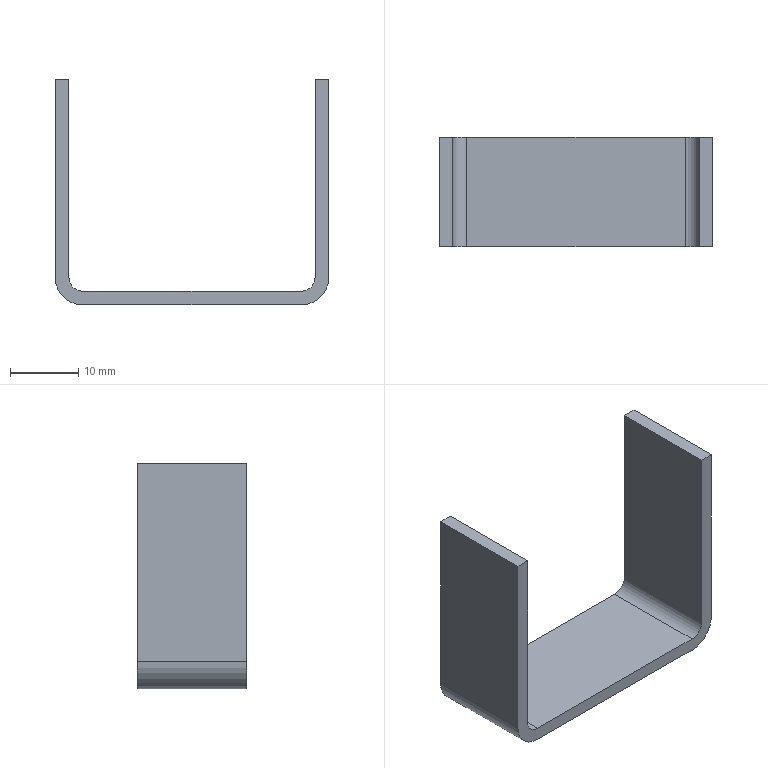Part | NX | features solid 2 | 1 solid | 14 faces | box 40 x 16 x 33 mm | volume 3182 mm3 | plane 10 | cylinder 4 | commonest cylinder face diameters 4 x2 8 x2
STEP:
#1=CARTESIAN_POINT('',(941.4,-1578.,922.));
#2=VERTEX_POINT('',#1);
#3=CARTESIAN_POINT('',(941.4,-1578.,951.));
#4=VERTEX_POINT('',#3);
#5=CARTESIAN_POINT('',(941.4,-1578.,918.));
#6=DIRECTION('',(0.,0.,1.));
#7=VECTOR('',#6,1000.);
#8=LINE('',#5,#7);
#9=EDGE_CURVE('',#2,#4,#8,.T.);
#10=ORIENTED_EDGE('',*,*,#9,.T.);
#11=CARTESIAN_POINT('',(941.4,-1562.,951.));
#12=VERTEX_POINT('',#11);
#13=CARTESIAN_POINT('',(941.4,-1562.,951.));
#14=DIRECTION('',(0.,-1.,0.));
#15=VECTOR('',#14,1000.);
#16=LINE('',#13,#15);
#17=EDGE_CURVE('',#12,#4,#16,.T.);
#18=ORIENTED_EDGE('',*,*,#17,.F.);
#19=CARTESIAN_POINT('',(941.4,-1562.,922.));
#20=VERTEX_POINT('',#19);
#21=CARTESIAN_POINT('',(941.4,-1562.,918.));
#22=DIRECTION('',(0.,0.,1.));
#23=VECTOR('',#22,1000.);
#24=LINE('',#21,#23);
#25=EDGE_CURVE('',#20,#12,#24,.T.);
#26=ORIENTED_EDGE('',*,*,#25,.F.);
#27=CARTESIAN_POINT('',(941.4,-1562.,922.));
#28=DIRECTION('',(0.,-1.,0.));
#29=VECTOR('',#28,1000.);
#30=LINE('',#27,#29);
#31=EDGE_CURVE('',#20,#2,#30,.T.);
#32=ORIENTED_EDGE('',*,*,#31,.T.);
#33=EDGE_LOOP('',(#10,#18,#26,#32));
#34=FACE_BOUND('',#33,.T.);
#35=CARTESIAN_POINT('',(941.4,-1562.,918.));
#36=DIRECTION('',(1.,0.,0.));
#37=DIRECTION('',(0.,1.,0.));
#38=AXIS2_PLACEMENT_3D('',#35,#36,#37);
#39=PLANE('',#38);
#40=ADVANCED_FACE('',(#34),#39,.F.);
#41=CARTESIAN_POINT('',(939.4,-1578.,920.));
#42=VERTEX_POINT('',#41);
#43=CARTESIAN_POINT('',(939.4,-1578.,922.));
#44=DIRECTION('',(0.,-1.,0.));
#45=DIRECTION('',(0.,0.,-1.));
#46=AXIS2_PLACEMENT_3D('',#43,#44,#45);
#47=CIRCLE('',#46,2.);
#48=EDGE_CURVE('',#42,#2,#47,.T.);
#49=ORIENTED_EDGE('',*,*,#48,.T.);
#50=ORIENTED_EDGE('',*,*,#31,.F.);
#51=CARTESIAN_POINT('',(939.4,-1562.,920.));
#52=VERTEX_POINT('',#51);
#53=CARTESIAN_POINT('',(939.4,-1562.,922.));
#54=DIRECTION('',(0.,-1.,0.));
#55=DIRECTION('',(0.,0.,-1.));
#56=AXIS2_PLACEMENT_3D('',#53,#54,#55);
#57=CIRCLE('',#56,2.);
#58=EDGE_CURVE('',#52,#20,#57,.T.);
#59=ORIENTED_EDGE('',*,*,#58,.F.);
#60=CARTESIAN_POINT('',(939.4,-1562.,920.));
#61=DIRECTION('',(0.,-1.,0.));
#62=VECTOR('',#61,1000.);
#63=LINE('',#60,#62);
#64=EDGE_CURVE('',#52,#42,#63,.T.);
#65=ORIENTED_EDGE('',*,*,#64,.T.);
#66=EDGE_LOOP('',(#49,#50,#59,#65));
#67=FACE_BOUND('',#66,.T.);
#68=CARTESIAN_POINT('',(939.4,-1562.,922.));
#69=DIRECTION('',(0.,-1.,0.));
#70=DIRECTION('',(0.,0.,-1.));
#71=AXIS2_PLACEMENT_3D('',#68,#69,#70);
#72=CYLINDRICAL_SURFACE('',#71,2.);
#73=ADVANCED_FACE('',(#67),#72,.F.);
#74=CARTESIAN_POINT('',(907.4,-1578.,920.));
#75=VERTEX_POINT('',#74);
#76=CARTESIAN_POINT('',(903.4,-1578.,920.));
#77=DIRECTION('',(1.,0.,0.));
#78=VECTOR('',#77,1000.);
#79=LINE('',#76,#78);
#80=EDGE_CURVE('',#75,#42,#79,.T.);
#81=ORIENTED_EDGE('',*,*,#80,.T.);
#82=ORIENTED_EDGE('',*,*,#64,.F.);
#83=CARTESIAN_POINT('',(907.4,-1562.,920.));
#84=VERTEX_POINT('',#83);
#85=CARTESIAN_POINT('',(903.4,-1562.,920.));
#86=DIRECTION('',(1.,0.,0.));
#87=VECTOR('',#86,1000.);
#88=LINE('',#85,#87);
#89=EDGE_CURVE('',#84,#52,#88,.T.);
#90=ORIENTED_EDGE('',*,*,#89,.F.);
#91=CARTESIAN_POINT('',(907.4,-1562.,920.));
#92=DIRECTION('',(0.,-1.,0.));
#93=VECTOR('',#92,1000.);
#94=LINE('',#91,#93);
#95=EDGE_CURVE('',#84,#75,#94,.T.);
#96=ORIENTED_EDGE('',*,*,#95,.T.);
#97=EDGE_LOOP('',(#81,#82,#90,#96));
#98=FACE_BOUND('',#97,.T.);
#99=CARTESIAN_POINT('',(903.4,-1562.,920.));
#100=DIRECTION('',(0.,0.,-1.));
#101=DIRECTION('',(0.,-1.,0.));
#102=AXIS2_PLACEMENT_3D('',#99,#100,#101);
#103=PLANE('',#102);
#104=ADVANCED_FACE('',(#98),#103,.F.);
#105=CARTESIAN_POINT('',(905.4,-1578.,922.));
#106=VERTEX_POINT('',#105);
#107=CARTESIAN_POINT('',(907.4,-1578.,922.));
#108=DIRECTION('',(0.,-1.,0.));
#109=DIRECTION('',(0.,0.,-1.));
#110=AXIS2_PLACEMENT_3D('',#107,#108,#109);
#111=CIRCLE('',#110,2.);
#112=EDGE_CURVE('',#106,#75,#111,.T.);
#113=ORIENTED_EDGE('',*,*,#112,.T.);
#114=ORIENTED_EDGE('',*,*,#95,.F.);
#115=CARTESIAN_POINT('',(905.4,-1562.,922.));
#116=VERTEX_POINT('',#115);
#117=CARTESIAN_POINT('',(907.4,-1562.,922.));
#118=DIRECTION('',(0.,-1.,0.));
#119=DIRECTION('',(0.,0.,-1.));
#120=AXIS2_PLACEMENT_3D('',#117,#118,#119);
#121=CIRCLE('',#120,2.);
#122=EDGE_CURVE('',#116,#84,#121,.T.);
#123=ORIENTED_EDGE('',*,*,#122,.F.);
#124=CARTESIAN_POINT('',(905.4,-1562.,922.));
#125=DIRECTION('',(0.,-1.,0.));
#126=VECTOR('',#125,1000.);
#127=LINE('',#124,#126);
#128=EDGE_CURVE('',#116,#106,#127,.T.);
#129=ORIENTED_EDGE('',*,*,#128,.T.);
#130=EDGE_LOOP('',(#113,#114,#123,#129));
#131=FACE_BOUND('',#130,.T.);
#132=CARTESIAN_POINT('',(907.4,-1562.,922.));
#133=DIRECTION('',(0.,-1.,0.));
#134=DIRECTION('',(0.,0.,-1.));
#135=AXIS2_PLACEMENT_3D('',#132,#133,#134);
#136=CYLINDRICAL_SURFACE('',#135,2.);
#137=ADVANCED_FACE('',(#131),#136,.F.);
#138=CARTESIAN_POINT('',(905.4,-1578.,951.));
#139=VERTEX_POINT('',#138);
#140=CARTESIAN_POINT('',(905.4,-1578.,951.));
#141=DIRECTION('',(0.,0.,-1.));
#142=VECTOR('',#141,1000.);
#143=LINE('',#140,#142);
#144=EDGE_CURVE('',#139,#106,#143,.T.);
#145=ORIENTED_EDGE('',*,*,#144,.T.);
#146=ORIENTED_EDGE('',*,*,#128,.F.);
#147=CARTESIAN_POINT('',(905.4,-1562.,951.));
#148=VERTEX_POINT('',#147);
#149=CARTESIAN_POINT('',(905.4,-1562.,951.));
#150=DIRECTION('',(0.,0.,-1.));
#151=VECTOR('',#150,1000.);
#152=LINE('',#149,#151);
#153=EDGE_CURVE('',#148,#116,#152,.T.);
#154=ORIENTED_EDGE('',*,*,#153,.F.);
#155=CARTESIAN_POINT('',(905.4,-1562.,951.));
#156=DIRECTION('',(0.,-1.,0.));
#157=VECTOR('',#156,1000.);
#158=LINE('',#155,#157);
#159=EDGE_CURVE('',#148,#139,#158,.T.);
#160=ORIENTED_EDGE('',*,*,#159,.T.);
#161=EDGE_LOOP('',(#145,#146,#154,#160));
#162=FACE_BOUND('',#161,.T.);
#163=CARTESIAN_POINT('',(905.4,-1562.,951.));
#164=DIRECTION('',(-1.,0.,0.));
#165=DIRECTION('',(0.,0.,1.));
#166=AXIS2_PLACEMENT_3D('',#163,#164,#165);
#167=PLANE('',#166);
#168=ADVANCED_FACE('',(#162),#167,.F.);
#169=CARTESIAN_POINT('',(943.4,-1578.,922.));
#170=VERTEX_POINT('',#169);
#171=CARTESIAN_POINT('',(943.4,-1578.,951.));
#172=VERTEX_POINT('',#171);
#173=CARTESIAN_POINT('',(943.4,-1578.,918.));
#174=DIRECTION('',(0.,0.,1.));
#175=VECTOR('',#174,1000.);
#176=LINE('',#173,#175);
#177=EDGE_CURVE('',#170,#172,#176,.T.);
#178=ORIENTED_EDGE('',*,*,#177,.F.);
#179=CARTESIAN_POINT('',(943.4,-1562.,922.));
#180=VERTEX_POINT('',#179);
#181=CARTESIAN_POINT('',(943.4,-1562.,922.));
#182=DIRECTION('',(0.,-1.,0.));
#183=VECTOR('',#182,1000.);
#184=LINE('',#181,#183);
#185=EDGE_CURVE('',#180,#170,#184,.T.);
#186=ORIENTED_EDGE('',*,*,#185,.F.);
#187=CARTESIAN_POINT('',(943.4,-1562.,951.));
#188=VERTEX_POINT('',#187);
#189=CARTESIAN_POINT('',(943.4,-1562.,918.));
#190=DIRECTION('',(0.,0.,1.));
#191=VECTOR('',#190,1000.);
#192=LINE('',#189,#191);
#193=EDGE_CURVE('',#180,#188,#192,.T.);
#194=ORIENTED_EDGE('',*,*,#193,.T.);
#195=CARTESIAN_POINT('',(943.4,-1562.,951.));
#196=DIRECTION('',(0.,-1.,0.));
#197=VECTOR('',#196,1000.);
#198=LINE('',#195,#197);
#199=EDGE_CURVE('',#188,#172,#198,.T.);
#200=ORIENTED_EDGE('',*,*,#199,.T.);
#201=EDGE_LOOP('',(#178,#186,#194,#200));
#202=FACE_BOUND('',#201,.T.);
#203=CARTESIAN_POINT('',(943.4,-1562.,918.));
#204=DIRECTION('',(1.,0.,0.));
#205=DIRECTION('',(0.,1.,0.));
#206=AXIS2_PLACEMENT_3D('',#203,#204,#205);
#207=PLANE('',#206);
#208=ADVANCED_FACE('',(#202),#207,.T.);
#209=CARTESIAN_POINT('',(939.4,-1578.,918.));
#210=VERTEX_POINT('',#209);
#211=CARTESIAN_POINT('',(939.4,-1578.,922.));
#212=DIRECTION('',(0.,-1.,0.));
#213=DIRECTION('',(0.,0.,1.));
#214=AXIS2_PLACEMENT_3D('',#211,#212,#213);
#215=CIRCLE('',#214,4.);
#216=EDGE_CURVE('',#210,#170,#215,.T.);
#217=ORIENTED_EDGE('',*,*,#216,.F.);
#218=CARTESIAN_POINT('',(939.4,-1562.,918.));
#219=VERTEX_POINT('',#218);
#220=CARTESIAN_POINT('',(939.4,-1562.,918.));
#221=DIRECTION('',(0.,-1.,0.));
#222=VECTOR('',#221,1000.);
#223=LINE('',#220,#222);
#224=EDGE_CURVE('',#219,#210,#223,.T.);
#225=ORIENTED_EDGE('',*,*,#224,.F.);
#226=CARTESIAN_POINT('',(939.4,-1562.,922.));
#227=DIRECTION('',(0.,-1.,0.));
#228=DIRECTION('',(0.,0.,1.));
#229=AXIS2_PLACEMENT_3D('',#226,#227,#228);
#230=CIRCLE('',#229,4.);
#231=EDGE_CURVE('',#219,#180,#230,.T.);
#232=ORIENTED_EDGE('',*,*,#231,.T.);
#233=ORIENTED_EDGE('',*,*,#185,.T.);
#234=EDGE_LOOP('',(#217,#225,#232,#233));
#235=FACE_BOUND('',#234,.T.);
#236=CARTESIAN_POINT('',(939.4,-1562.,922.));
#237=DIRECTION('',(0.,-1.,0.));
#238=DIRECTION('',(0.,0.,-1.));
#239=AXIS2_PLACEMENT_3D('',#236,#237,#238);
#240=CYLINDRICAL_SURFACE('',#239,4.);
#241=ADVANCED_FACE('',(#235),#240,.T.);
#242=CARTESIAN_POINT('',(907.4,-1578.,918.));
#243=VERTEX_POINT('',#242);
#244=CARTESIAN_POINT('',(903.4,-1578.,918.));
#245=DIRECTION('',(1.,0.,0.));
#246=VECTOR('',#245,1000.);
#247=LINE('',#244,#246);
#248=EDGE_CURVE('',#243,#210,#247,.T.);
#249=ORIENTED_EDGE('',*,*,#248,.F.);
#250=CARTESIAN_POINT('',(907.4,-1562.,918.));
#251=VERTEX_POINT('',#250);
#252=CARTESIAN_POINT('',(907.4,-1562.,918.));
#253=DIRECTION('',(0.,-1.,0.));
#254=VECTOR('',#253,1000.);
#255=LINE('',#252,#254);
#256=EDGE_CURVE('',#251,#243,#255,.T.);
#257=ORIENTED_EDGE('',*,*,#256,.F.);
#258=CARTESIAN_POINT('',(903.4,-1562.,918.));
#259=DIRECTION('',(1.,0.,0.));
#260=VECTOR('',#259,1000.);
#261=LINE('',#258,#260);
#262=EDGE_CURVE('',#251,#219,#261,.T.);
#263=ORIENTED_EDGE('',*,*,#262,.T.);
#264=ORIENTED_EDGE('',*,*,#224,.T.);
#265=EDGE_LOOP('',(#249,#257,#263,#264));
#266=FACE_BOUND('',#265,.T.);
#267=CARTESIAN_POINT('',(903.4,-1562.,918.));
#268=DIRECTION('',(0.,0.,-1.));
#269=DIRECTION('',(0.,-1.,0.));
#270=AXIS2_PLACEMENT_3D('',#267,#268,#269);
#271=PLANE('',#270);
#272=ADVANCED_FACE('',(#266),#271,.T.);
#273=CARTESIAN_POINT('',(903.4,-1578.,922.));
#274=VERTEX_POINT('',#273);
#275=CARTESIAN_POINT('',(907.4,-1578.,922.));
#276=DIRECTION('',(0.,-1.,0.));
#277=DIRECTION('',(0.,0.,1.));
#278=AXIS2_PLACEMENT_3D('',#275,#276,#277);
#279=CIRCLE('',#278,4.);
#280=EDGE_CURVE('',#274,#243,#279,.T.);
#281=ORIENTED_EDGE('',*,*,#280,.F.);
#282=CARTESIAN_POINT('',(903.4,-1562.,922.));
#283=VERTEX_POINT('',#282);
#284=CARTESIAN_POINT('',(903.4,-1562.,922.));
#285=DIRECTION('',(0.,-1.,0.));
#286=VECTOR('',#285,1000.);
#287=LINE('',#284,#286);
#288=EDGE_CURVE('',#283,#274,#287,.T.);
#289=ORIENTED_EDGE('',*,*,#288,.F.);
#290=CARTESIAN_POINT('',(907.4,-1562.,922.));
#291=DIRECTION('',(0.,-1.,0.));
#292=DIRECTION('',(0.,0.,1.));
#293=AXIS2_PLACEMENT_3D('',#290,#291,#292);
#294=CIRCLE('',#293,4.);
#295=EDGE_CURVE('',#283,#251,#294,.T.);
#296=ORIENTED_EDGE('',*,*,#295,.T.);
#297=ORIENTED_EDGE('',*,*,#256,.T.);
#298=EDGE_LOOP('',(#281,#289,#296,#297));
#299=FACE_BOUND('',#298,.T.);
#300=CARTESIAN_POINT('',(907.4,-1562.,922.));
#301=DIRECTION('',(0.,-1.,0.));
#302=DIRECTION('',(0.,0.,-1.));
#303=AXIS2_PLACEMENT_3D('',#300,#301,#302);
#304=CYLINDRICAL_SURFACE('',#303,4.);
#305=ADVANCED_FACE('',(#299),#304,.T.);
#306=CARTESIAN_POINT('',(903.4,-1578.,951.));
#307=VERTEX_POINT('',#306);
#308=CARTESIAN_POINT('',(903.4,-1578.,951.));
#309=DIRECTION('',(0.,0.,-1.));
#310=VECTOR('',#309,1000.);
#311=LINE('',#308,#310);
#312=EDGE_CURVE('',#307,#274,#311,.T.);
#313=ORIENTED_EDGE('',*,*,#312,.F.);
#314=CARTESIAN_POINT('',(903.4,-1562.,951.));
#315=VERTEX_POINT('',#314);
#316=CARTESIAN_POINT('',(903.4,-1562.,951.));
#317=DIRECTION('',(0.,-1.,0.));
#318=VECTOR('',#317,1000.);
#319=LINE('',#316,#318);
#320=EDGE_CURVE('',#315,#307,#319,.T.);
#321=ORIENTED_EDGE('',*,*,#320,.F.);
#322=CARTESIAN_POINT('',(903.4,-1562.,951.));
#323=DIRECTION('',(0.,0.,-1.));
#324=VECTOR('',#323,1000.);
#325=LINE('',#322,#324);
#326=EDGE_CURVE('',#315,#283,#325,.T.);
#327=ORIENTED_EDGE('',*,*,#326,.T.);
#328=ORIENTED_EDGE('',*,*,#288,.T.);
#329=EDGE_LOOP('',(#313,#321,#327,#328));
#330=FACE_BOUND('',#329,.T.);
#331=CARTESIAN_POINT('',(903.4,-1562.,951.));
#332=DIRECTION('',(-1.,0.,0.));
#333=DIRECTION('',(0.,0.,1.));
#334=AXIS2_PLACEMENT_3D('',#331,#332,#333);
#335=PLANE('',#334);
#336=ADVANCED_FACE('',(#330),#335,.T.);
#337=ORIENTED_EDGE('',*,*,#159,.F.);
#338=CARTESIAN_POINT('',(903.4,-1562.,951.));
#339=DIRECTION('',(-1.,0.,0.));
#340=VECTOR('',#339,1000.);
#341=LINE('',#338,#340);
#342=EDGE_CURVE('',#148,#315,#341,.T.);
#343=ORIENTED_EDGE('',*,*,#342,.T.);
#344=ORIENTED_EDGE('',*,*,#320,.T.);
#345=CARTESIAN_POINT('',(903.4,-1578.,951.));
#346=DIRECTION('',(-1.,0.,0.));
#347=VECTOR('',#346,1000.);
#348=LINE('',#345,#347);
#349=EDGE_CURVE('',#139,#307,#348,.T.);
#350=ORIENTED_EDGE('',*,*,#349,.F.);
#351=EDGE_LOOP('',(#337,#343,#344,#350));
#352=FACE_BOUND('',#351,.T.);
#353=CARTESIAN_POINT('',(903.4,-1562.,951.));
#354=DIRECTION('',(0.,0.,-1.));
#355=DIRECTION('',(0.,-1.,0.));
#356=AXIS2_PLACEMENT_3D('',#353,#354,#355);
#357=PLANE('',#356);
#358=ADVANCED_FACE('',(#352),#357,.F.);
#359=ORIENTED_EDGE('',*,*,#312,.T.);
#360=ORIENTED_EDGE('',*,*,#280,.T.);
#361=ORIENTED_EDGE('',*,*,#248,.T.);
#362=ORIENTED_EDGE('',*,*,#216,.T.);
#363=ORIENTED_EDGE('',*,*,#177,.T.);
#364=CARTESIAN_POINT('',(943.4,-1578.,951.));
#365=DIRECTION('',(1.,0.,0.));
#366=VECTOR('',#365,1000.);
#367=LINE('',#364,#366);
#368=EDGE_CURVE('',#4,#172,#367,.T.);
#369=ORIENTED_EDGE('',*,*,#368,.F.);
#370=ORIENTED_EDGE('',*,*,#9,.F.);
#371=ORIENTED_EDGE('',*,*,#48,.F.);
#372=ORIENTED_EDGE('',*,*,#80,.F.);
#373=ORIENTED_EDGE('',*,*,#112,.F.);
#374=ORIENTED_EDGE('',*,*,#144,.F.);
#375=ORIENTED_EDGE('',*,*,#349,.T.);
#376=EDGE_LOOP('',(#359,#360,#361,#362,#363,#369,#370,#371,#372,#373,#374,#375));
#377=FACE_BOUND('',#376,.T.);
#378=CARTESIAN_POINT('',(903.4,-1578.,951.));
#379=DIRECTION('',(0.,1.,0.));
#380=DIRECTION('',(1.,0.,0.));
#381=AXIS2_PLACEMENT_3D('',#378,#379,#380);
#382=PLANE('',#381);
#383=ADVANCED_FACE('',(#377),#382,.F.);
#384=CARTESIAN_POINT('',(943.4,-1562.,951.));
#385=DIRECTION('',(1.,0.,0.));
#386=VECTOR('',#385,1000.);
#387=LINE('',#384,#386);
#388=EDGE_CURVE('',#12,#188,#387,.T.);
#389=ORIENTED_EDGE('',*,*,#388,.F.);
#390=ORIENTED_EDGE('',*,*,#17,.T.);
#391=ORIENTED_EDGE('',*,*,#368,.T.);
#392=ORIENTED_EDGE('',*,*,#199,.F.);
#393=EDGE_LOOP('',(#389,#390,#391,#392));
#394=FACE_BOUND('',#393,.T.);
#395=CARTESIAN_POINT('',(943.4,-1562.,951.));
#396=DIRECTION('',(0.,0.,1.));
#397=DIRECTION('',(1.,0.,0.));
#398=AXIS2_PLACEMENT_3D('',#395,#396,#397);
#399=PLANE('',#398);
#400=ADVANCED_FACE('',(#394),#399,.T.);
#401=ORIENTED_EDGE('',*,*,#193,.F.);
#402=ORIENTED_EDGE('',*,*,#231,.F.);
#403=ORIENTED_EDGE('',*,*,#262,.F.);
#404=ORIENTED_EDGE('',*,*,#295,.F.);
#405=ORIENTED_EDGE('',*,*,#326,.F.);
#406=ORIENTED_EDGE('',*,*,#342,.F.);
#407=ORIENTED_EDGE('',*,*,#153,.T.);
#408=ORIENTED_EDGE('',*,*,#122,.T.);
#409=ORIENTED_EDGE('',*,*,#89,.T.);
#410=ORIENTED_EDGE('',*,*,#58,.T.);
#411=ORIENTED_EDGE('',*,*,#25,.T.);
#412=ORIENTED_EDGE('',*,*,#388,.T.);
#413=EDGE_LOOP('',(#401,#402,#403,#404,#405,#406,#407,#408,#409,#410,#411,#412));
#414=FACE_BOUND('',#413,.T.);
#415=CARTESIAN_POINT('',(943.4,-1562.,918.));
#416=DIRECTION('',(0.,1.,0.));
#417=DIRECTION('',(1.,0.,0.));
#418=AXIS2_PLACEMENT_3D('',#415,#416,#417);
#419=PLANE('',#418);
#420=ADVANCED_FACE('',(#414),#419,.T.);
#421=CLOSED_SHELL('',(#40,#73,#104,#137,#168,#208,#241,#272,#305,#336,#358,#383,#400,#420));
#422=MANIFOLD_SOLID_BREP('',#421);
#423=(LENGTH_UNIT()NAMED_UNIT(*)SI_UNIT(.MILLI.,.METRE.));
#424=UNCERTAINTY_MEASURE_WITH_UNIT(LENGTH_MEASURE(0.00001),#423,'','');
#425=(NAMED_UNIT(*)PLANE_ANGLE_UNIT()SI_UNIT($,.RADIAN.));
#426=(NAMED_UNIT(*)SI_UNIT($,.STERADIAN.)SOLID_ANGLE_UNIT());
#427=(GEOMETRIC_REPRESENTATION_CONTEXT(3)GLOBAL_UNCERTAINTY_ASSIGNED_CONTEXT((#424))GLOBAL_UNIT_ASSIGNED_CONTEXT((#423,#425,#426))REPRESENTATION_CONTEXT('',''));
#428=ADVANCED_BREP_SHAPE_REPRESENTATION('',(#422),#427);